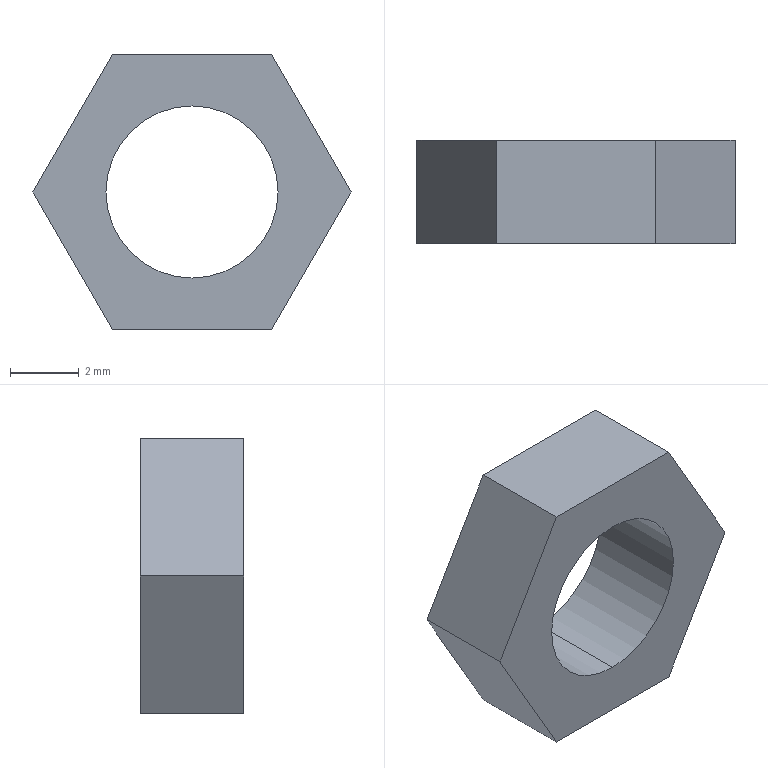Part | NX | features BREP 1 | 1 solid | 10 faces | box 9.238 x 3 x 8 mm | volume 107.372 mm3 | plane 8 | cylinder 2 | commonest cylinder face diameters 5 x2
STEP:
#1=CARTESIAN_POINT('',(0.,3.,-2.5));
#2=VERTEX_POINT('',#1);
#3=CARTESIAN_POINT('',(0.,3.,2.5));
#4=VERTEX_POINT('',#3);
#5=CARTESIAN_POINT('',(0.,3.,0.));
#6=DIRECTION('',(0.,1.,0.));
#7=DIRECTION('',(0.,0.,1.));
#8=AXIS2_PLACEMENT_3D('',#5,#6,#7);
#9=CIRCLE('',#8,2.5);
#10=EDGE_CURVE('',#2,#4,#9,.T.);
#11=ORIENTED_EDGE('',*,*,#10,.T.);
#12=CARTESIAN_POINT('',(0.,0.,2.5));
#13=VERTEX_POINT('',#12);
#14=CARTESIAN_POINT('',(0.,3.,2.5));
#15=DIRECTION('',(0.,-1.,0.));
#16=VECTOR('',#15,1000.);
#17=LINE('',#14,#16);
#18=EDGE_CURVE('',#13,#4,#17,.F.);
#19=ORIENTED_EDGE('',*,*,#18,.F.);
#20=CARTESIAN_POINT('',(0.,0.,-2.5));
#21=VERTEX_POINT('',#20);
#22=CARTESIAN_POINT('',(0.,0.,0.));
#23=DIRECTION('',(0.,1.,0.));
#24=DIRECTION('',(0.,0.,1.));
#25=AXIS2_PLACEMENT_3D('',#22,#23,#24);
#26=CIRCLE('',#25,2.5);
#27=EDGE_CURVE('',#21,#13,#26,.T.);
#28=ORIENTED_EDGE('',*,*,#27,.F.);
#29=CARTESIAN_POINT('',(0.,3.,-2.5));
#30=DIRECTION('',(0.,-1.,0.));
#31=VECTOR('',#30,1000.);
#32=LINE('',#29,#31);
#33=EDGE_CURVE('',#21,#2,#32,.F.);
#34=ORIENTED_EDGE('',*,*,#33,.T.);
#35=EDGE_LOOP('',(#11,#19,#28,#34));
#36=FACE_BOUND('',#35,.T.);
#37=CARTESIAN_POINT('',(0.,3.,0.));
#38=DIRECTION('',(0.,-1.,0.));
#39=DIRECTION('',(0.,0.,1.));
#40=AXIS2_PLACEMENT_3D('',#37,#38,#39);
#41=CYLINDRICAL_SURFACE('',#40,2.5);
#42=ADVANCED_FACE('',(#36),#41,.F.);
#43=CARTESIAN_POINT('',(2.309,3.,4.));
#44=VERTEX_POINT('',#43);
#45=CARTESIAN_POINT('',(4.619,3.,0.));
#46=VERTEX_POINT('',#45);
#47=CARTESIAN_POINT('',(2.309,3.,4.));
#48=DIRECTION('',(0.5,0.,-0.866));
#49=VECTOR('',#48,1000.);
#50=LINE('',#47,#49);
#51=EDGE_CURVE('',#44,#46,#50,.T.);
#52=ORIENTED_EDGE('',*,*,#51,.T.);
#53=CARTESIAN_POINT('',(2.309,3.,-4.));
#54=VERTEX_POINT('',#53);
#55=CARTESIAN_POINT('',(4.619,3.,0.));
#56=DIRECTION('',(-0.5,0.,-0.866));
#57=VECTOR('',#56,1000.);
#58=LINE('',#55,#57);
#59=EDGE_CURVE('',#46,#54,#58,.T.);
#60=ORIENTED_EDGE('',*,*,#59,.T.);
#61=CARTESIAN_POINT('',(-2.309,3.,-4.));
#62=VERTEX_POINT('',#61);
#63=CARTESIAN_POINT('',(2.309,3.,-4.));
#64=DIRECTION('',(-1.,0.,0.));
#65=VECTOR('',#64,1000.);
#66=LINE('',#63,#65);
#67=EDGE_CURVE('',#54,#62,#66,.T.);
#68=ORIENTED_EDGE('',*,*,#67,.T.);
#69=CARTESIAN_POINT('',(-4.619,3.,0.));
#70=VERTEX_POINT('',#69);
#71=CARTESIAN_POINT('',(-2.309,3.,-4.));
#72=DIRECTION('',(-0.5,0.,0.866));
#73=VECTOR('',#72,1000.);
#74=LINE('',#71,#73);
#75=EDGE_CURVE('',#62,#70,#74,.T.);
#76=ORIENTED_EDGE('',*,*,#75,.T.);
#77=CARTESIAN_POINT('',(-2.309,3.,4.));
#78=VERTEX_POINT('',#77);
#79=CARTESIAN_POINT('',(-4.619,3.,0.));
#80=DIRECTION('',(0.5,0.,0.866));
#81=VECTOR('',#80,1000.);
#82=LINE('',#79,#81);
#83=EDGE_CURVE('',#70,#78,#82,.T.);
#84=ORIENTED_EDGE('',*,*,#83,.T.);
#85=CARTESIAN_POINT('',(-2.309,3.,4.));
#86=DIRECTION('',(1.,0.,0.));
#87=VECTOR('',#86,1000.);
#88=LINE('',#85,#87);
#89=EDGE_CURVE('',#78,#44,#88,.T.);
#90=ORIENTED_EDGE('',*,*,#89,.T.);
#91=EDGE_LOOP('',(#52,#60,#68,#76,#84,#90));
#92=FACE_BOUND('',#91,.T.);
#93=ORIENTED_EDGE('',*,*,#10,.F.);
#94=CARTESIAN_POINT('',(0.,3.,0.));
#95=DIRECTION('',(0.,1.,0.));
#96=DIRECTION('',(0.,0.,1.));
#97=AXIS2_PLACEMENT_3D('',#94,#95,#96);
#98=CIRCLE('',#97,2.5);
#99=EDGE_CURVE('',#4,#2,#98,.T.);
#100=ORIENTED_EDGE('',*,*,#99,.F.);
#101=EDGE_LOOP('',(#93,#100));
#102=FACE_BOUND('',#101,.T.);
#103=CARTESIAN_POINT('',(0.,3.,0.));
#104=DIRECTION('',(0.,1.,0.));
#105=DIRECTION('',(0.,0.,1.));
#106=AXIS2_PLACEMENT_3D('',#103,#104,#105);
#107=PLANE('',#106);
#108=ADVANCED_FACE('',(#92,#102),#107,.T.);
#109=CARTESIAN_POINT('',(2.309,0.,4.));
#110=VERTEX_POINT('',#109);
#111=CARTESIAN_POINT('',(4.619,0.,0.));
#112=VERTEX_POINT('',#111);
#113=CARTESIAN_POINT('',(2.309,0.,4.));
#114=DIRECTION('',(0.5,0.,-0.866));
#115=VECTOR('',#114,1000.);
#116=LINE('',#113,#115);
#117=EDGE_CURVE('',#110,#112,#116,.T.);
#118=ORIENTED_EDGE('',*,*,#117,.F.);
#119=CARTESIAN_POINT('',(-2.309,0.,4.));
#120=VERTEX_POINT('',#119);
#121=CARTESIAN_POINT('',(-2.309,0.,4.));
#122=DIRECTION('',(1.,0.,0.));
#123=VECTOR('',#122,1000.);
#124=LINE('',#121,#123);
#125=EDGE_CURVE('',#120,#110,#124,.T.);
#126=ORIENTED_EDGE('',*,*,#125,.F.);
#127=CARTESIAN_POINT('',(-4.619,0.,0.));
#128=VERTEX_POINT('',#127);
#129=CARTESIAN_POINT('',(-4.619,0.,0.));
#130=DIRECTION('',(0.5,0.,0.866));
#131=VECTOR('',#130,1000.);
#132=LINE('',#129,#131);
#133=EDGE_CURVE('',#128,#120,#132,.T.);
#134=ORIENTED_EDGE('',*,*,#133,.F.);
#135=CARTESIAN_POINT('',(-2.309,0.,-4.));
#136=VERTEX_POINT('',#135);
#137=CARTESIAN_POINT('',(-2.309,0.,-4.));
#138=DIRECTION('',(-0.5,0.,0.866));
#139=VECTOR('',#138,1000.);
#140=LINE('',#137,#139);
#141=EDGE_CURVE('',#136,#128,#140,.T.);
#142=ORIENTED_EDGE('',*,*,#141,.F.);
#143=CARTESIAN_POINT('',(2.309,0.,-4.));
#144=VERTEX_POINT('',#143);
#145=CARTESIAN_POINT('',(2.309,0.,-4.));
#146=DIRECTION('',(-1.,0.,0.));
#147=VECTOR('',#146,1000.);
#148=LINE('',#145,#147);
#149=EDGE_CURVE('',#144,#136,#148,.T.);
#150=ORIENTED_EDGE('',*,*,#149,.F.);
#151=CARTESIAN_POINT('',(4.619,0.,0.));
#152=DIRECTION('',(-0.5,0.,-0.866));
#153=VECTOR('',#152,1000.);
#154=LINE('',#151,#153);
#155=EDGE_CURVE('',#112,#144,#154,.T.);
#156=ORIENTED_EDGE('',*,*,#155,.F.);
#157=EDGE_LOOP('',(#118,#126,#134,#142,#150,#156));
#158=FACE_BOUND('',#157,.T.);
#159=ORIENTED_EDGE('',*,*,#27,.T.);
#160=CARTESIAN_POINT('',(0.,0.,0.));
#161=DIRECTION('',(0.,1.,0.));
#162=DIRECTION('',(0.,0.,1.));
#163=AXIS2_PLACEMENT_3D('',#160,#161,#162);
#164=CIRCLE('',#163,2.5);
#165=EDGE_CURVE('',#13,#21,#164,.T.);
#166=ORIENTED_EDGE('',*,*,#165,.T.);
#167=EDGE_LOOP('',(#159,#166));
#168=FACE_BOUND('',#167,.T.);
#169=CARTESIAN_POINT('',(0.,0.,0.));
#170=DIRECTION('',(0.,1.,0.));
#171=DIRECTION('',(0.,0.,1.));
#172=AXIS2_PLACEMENT_3D('',#169,#170,#171);
#173=PLANE('',#172);
#174=ADVANCED_FACE('',(#158,#168),#173,.F.);
#175=ORIENTED_EDGE('',*,*,#117,.T.);
#176=CARTESIAN_POINT('',(4.619,3.,0.));
#177=DIRECTION('',(0.,-1.,0.));
#178=VECTOR('',#177,1000.);
#179=LINE('',#176,#178);
#180=EDGE_CURVE('',#46,#112,#179,.T.);
#181=ORIENTED_EDGE('',*,*,#180,.F.);
#182=ORIENTED_EDGE('',*,*,#51,.F.);
#183=CARTESIAN_POINT('',(2.309,3.,4.));
#184=DIRECTION('',(0.,-1.,0.));
#185=VECTOR('',#184,1000.);
#186=LINE('',#183,#185);
#187=EDGE_CURVE('',#44,#110,#186,.T.);
#188=ORIENTED_EDGE('',*,*,#187,.T.);
#189=EDGE_LOOP('',(#175,#181,#182,#188));
#190=FACE_BOUND('',#189,.T.);
#191=CARTESIAN_POINT('',(2.309,3.,4.));
#192=DIRECTION('',(-0.866,0.,-0.5));
#193=DIRECTION('',(0.5,0.,-0.866));
#194=AXIS2_PLACEMENT_3D('',#191,#192,#193);
#195=PLANE('',#194);
#196=ADVANCED_FACE('',(#190),#195,.F.);
#197=ORIENTED_EDGE('',*,*,#155,.T.);
#198=CARTESIAN_POINT('',(2.309,3.,-4.));
#199=DIRECTION('',(0.,-1.,0.));
#200=VECTOR('',#199,1000.);
#201=LINE('',#198,#200);
#202=EDGE_CURVE('',#54,#144,#201,.T.);
#203=ORIENTED_EDGE('',*,*,#202,.F.);
#204=ORIENTED_EDGE('',*,*,#59,.F.);
#205=ORIENTED_EDGE('',*,*,#180,.T.);
#206=EDGE_LOOP('',(#197,#203,#204,#205));
#207=FACE_BOUND('',#206,.T.);
#208=CARTESIAN_POINT('',(4.619,3.,0.));
#209=DIRECTION('',(-0.866,0.,0.5));
#210=DIRECTION('',(0.,-1.,0.));
#211=AXIS2_PLACEMENT_3D('',#208,#209,#210);
#212=PLANE('',#211);
#213=ADVANCED_FACE('',(#207),#212,.F.);
#214=ORIENTED_EDGE('',*,*,#149,.T.);
#215=CARTESIAN_POINT('',(-2.309,3.,-4.));
#216=DIRECTION('',(0.,-1.,0.));
#217=VECTOR('',#216,1000.);
#218=LINE('',#215,#217);
#219=EDGE_CURVE('',#62,#136,#218,.T.);
#220=ORIENTED_EDGE('',*,*,#219,.F.);
#221=ORIENTED_EDGE('',*,*,#67,.F.);
#222=ORIENTED_EDGE('',*,*,#202,.T.);
#223=EDGE_LOOP('',(#214,#220,#221,#222));
#224=FACE_BOUND('',#223,.T.);
#225=CARTESIAN_POINT('',(2.309,3.,-4.));
#226=DIRECTION('',(0.,0.,1.));
#227=DIRECTION('',(-1.,0.,0.));
#228=AXIS2_PLACEMENT_3D('',#225,#226,#227);
#229=PLANE('',#228);
#230=ADVANCED_FACE('',(#224),#229,.F.);
#231=ORIENTED_EDGE('',*,*,#141,.T.);
#232=CARTESIAN_POINT('',(-4.619,3.,0.));
#233=DIRECTION('',(0.,-1.,0.));
#234=VECTOR('',#233,1000.);
#235=LINE('',#232,#234);
#236=EDGE_CURVE('',#70,#128,#235,.T.);
#237=ORIENTED_EDGE('',*,*,#236,.F.);
#238=ORIENTED_EDGE('',*,*,#75,.F.);
#239=ORIENTED_EDGE('',*,*,#219,.T.);
#240=EDGE_LOOP('',(#231,#237,#238,#239));
#241=FACE_BOUND('',#240,.T.);
#242=CARTESIAN_POINT('',(-2.309,3.,-4.));
#243=DIRECTION('',(0.866,0.,0.5));
#244=DIRECTION('',(0.,1.,0.));
#245=AXIS2_PLACEMENT_3D('',#242,#243,#244);
#246=PLANE('',#245);
#247=ADVANCED_FACE('',(#241),#246,.F.);
#248=ORIENTED_EDGE('',*,*,#133,.T.);
#249=CARTESIAN_POINT('',(-2.309,3.,4.));
#250=DIRECTION('',(0.,-1.,0.));
#251=VECTOR('',#250,1000.);
#252=LINE('',#249,#251);
#253=EDGE_CURVE('',#78,#120,#252,.T.);
#254=ORIENTED_EDGE('',*,*,#253,.F.);
#255=ORIENTED_EDGE('',*,*,#83,.F.);
#256=ORIENTED_EDGE('',*,*,#236,.T.);
#257=EDGE_LOOP('',(#248,#254,#255,#256));
#258=FACE_BOUND('',#257,.T.);
#259=CARTESIAN_POINT('',(-4.619,3.,0.));
#260=DIRECTION('',(0.866,0.,-0.5));
#261=DIRECTION('',(0.,1.,0.));
#262=AXIS2_PLACEMENT_3D('',#259,#260,#261);
#263=PLANE('',#262);
#264=ADVANCED_FACE('',(#258),#263,.F.);
#265=ORIENTED_EDGE('',*,*,#125,.T.);
#266=ORIENTED_EDGE('',*,*,#187,.F.);
#267=ORIENTED_EDGE('',*,*,#89,.F.);
#268=ORIENTED_EDGE('',*,*,#253,.T.);
#269=EDGE_LOOP('',(#265,#266,#267,#268));
#270=FACE_BOUND('',#269,.T.);
#271=CARTESIAN_POINT('',(-2.309,3.,4.));
#272=DIRECTION('',(0.,0.,-1.));
#273=DIRECTION('',(1.,0.,0.));
#274=AXIS2_PLACEMENT_3D('',#271,#272,#273);
#275=PLANE('',#274);
#276=ADVANCED_FACE('',(#270),#275,.F.);
#277=ORIENTED_EDGE('',*,*,#18,.T.);
#278=ORIENTED_EDGE('',*,*,#99,.T.);
#279=ORIENTED_EDGE('',*,*,#33,.F.);
#280=ORIENTED_EDGE('',*,*,#165,.F.);
#281=EDGE_LOOP('',(#277,#278,#279,#280));
#282=FACE_BOUND('',#281,.T.);
#283=CARTESIAN_POINT('',(0.,3.,0.));
#284=DIRECTION('',(0.,-1.,0.));
#285=DIRECTION('',(0.,0.,1.));
#286=AXIS2_PLACEMENT_3D('',#283,#284,#285);
#287=CYLINDRICAL_SURFACE('',#286,2.5);
#288=ADVANCED_FACE('',(#282),#287,.F.);
#289=CLOSED_SHELL('',(#42,#108,#174,#196,#213,#230,#247,#264,#276,#288));
#290=MANIFOLD_SOLID_BREP('',#289);
#291=(LENGTH_UNIT()NAMED_UNIT(*)SI_UNIT(.MILLI.,.METRE.));
#292=UNCERTAINTY_MEASURE_WITH_UNIT(LENGTH_MEASURE(0.00001),#291,'','');
#293=(NAMED_UNIT(*)PLANE_ANGLE_UNIT()SI_UNIT($,.RADIAN.));
#294=(NAMED_UNIT(*)SI_UNIT($,.STERADIAN.)SOLID_ANGLE_UNIT());
#295=(GEOMETRIC_REPRESENTATION_CONTEXT(3)GLOBAL_UNCERTAINTY_ASSIGNED_CONTEXT((#292))GLOBAL_UNIT_ASSIGNED_CONTEXT((#291,#293,#294))REPRESENTATION_CONTEXT('',''));
#296=ADVANCED_BREP_SHAPE_REPRESENTATION('',(#290),#295);